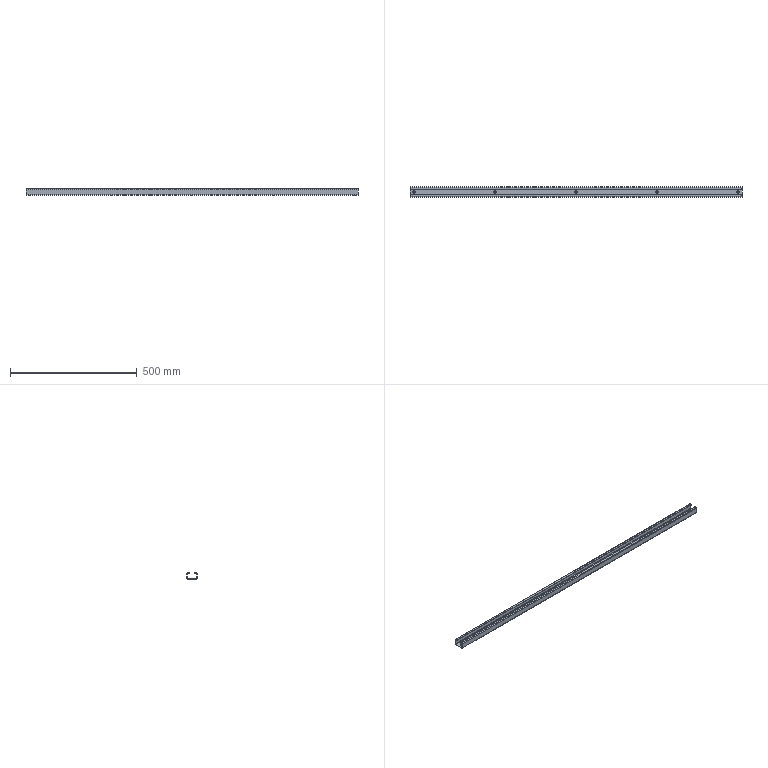Part | NX | features solid 2 | 1 solid | 36 faces | box 1310 x 39.5 x 25.5 mm | volume 197290 mm3 | plane 14 | cylinder 12 | cone 10 | commonest cylinder face diameters 3 x4 6 x4 10 x4
STEP:
#1=CARTESIAN_POINT('',(-273.5,-1500.5,1297.5));
#2=VERTEX_POINT('',#1);
#3=CARTESIAN_POINT('',(-268.5,-1505.5,1297.5));
#4=VERTEX_POINT('',#3);
#5=CARTESIAN_POINT('',(-268.5,-1500.5,1297.5));
#6=DIRECTION('',(0.,0.,1.));
#7=DIRECTION('',(0.,1.,0.));
#8=AXIS2_PLACEMENT_3D('',#5,#6,#7);
#9=CIRCLE('',#8,5.);
#10=EDGE_CURVE('',#2,#4,#9,.T.);
#11=ORIENTED_EDGE('',*,*,#10,.F.);
#12=CARTESIAN_POINT('',(-273.5,-1500.5,1296.));
#13=VERTEX_POINT('',#12);
#14=CARTESIAN_POINT('',(-273.5,-1500.5,1297.5));
#15=DIRECTION('',(0.,0.,1.));
#16=VECTOR('',#15,1000.);
#17=LINE('',#14,#16);
#18=EDGE_CURVE('',#13,#2,#17,.T.);
#19=ORIENTED_EDGE('',*,*,#18,.F.);
#20=CARTESIAN_POINT('',(-268.5,-1505.5,1296.));
#21=VERTEX_POINT('',#20);
#22=CARTESIAN_POINT('',(-268.5,-1500.5,1296.));
#23=DIRECTION('',(0.,0.,-1.));
#24=DIRECTION('',(0.,1.,0.));
#25=AXIS2_PLACEMENT_3D('',#22,#23,#24);
#26=CIRCLE('',#25,5.);
#27=EDGE_CURVE('',#21,#13,#26,.T.);
#28=ORIENTED_EDGE('',*,*,#27,.F.);
#29=CARTESIAN_POINT('',(-268.5,-1505.5,1297.5));
#30=DIRECTION('',(0.,0.,-1.));
#31=VECTOR('',#30,1000.);
#32=LINE('',#29,#31);
#33=EDGE_CURVE('',#4,#21,#32,.T.);
#34=ORIENTED_EDGE('',*,*,#33,.F.);
#35=EDGE_LOOP('',(#11,#19,#28,#34));
#36=FACE_BOUND('',#35,.T.);
#37=CARTESIAN_POINT('',(-268.5,-1500.5,1297.5));
#38=DIRECTION('',(0.,0.,1.));
#39=DIRECTION('',(0.,-1.,0.));
#40=AXIS2_PLACEMENT_3D('',#37,#38,#39);
#41=CYLINDRICAL_SURFACE('',#40,5.);
#42=ADVANCED_FACE('',(#36),#41,.T.);
#43=CARTESIAN_POINT('',(-268.5,-1525.,1297.5));
#44=VERTEX_POINT('',#43);
#45=CARTESIAN_POINT('',(-273.5,-1530.,1297.5));
#46=VERTEX_POINT('',#45);
#47=CARTESIAN_POINT('',(-268.5,-1530.,1297.5));
#48=DIRECTION('',(0.,0.,1.));
#49=DIRECTION('',(0.,1.,0.));
#50=AXIS2_PLACEMENT_3D('',#47,#48,#49);
#51=CIRCLE('',#50,5.);
#52=EDGE_CURVE('',#44,#46,#51,.T.);
#53=ORIENTED_EDGE('',*,*,#52,.F.);
#54=CARTESIAN_POINT('',(-268.5,-1525.,1296.));
#55=VERTEX_POINT('',#54);
#56=CARTESIAN_POINT('',(-268.5,-1525.,1297.5));
#57=DIRECTION('',(0.,0.,1.));
#58=VECTOR('',#57,1000.);
#59=LINE('',#56,#58);
#60=EDGE_CURVE('',#55,#44,#59,.T.);
#61=ORIENTED_EDGE('',*,*,#60,.F.);
#62=CARTESIAN_POINT('',(-273.5,-1530.,1296.));
#63=VERTEX_POINT('',#62);
#64=CARTESIAN_POINT('',(-268.5,-1530.,1296.));
#65=DIRECTION('',(0.,0.,-1.));
#66=DIRECTION('',(0.,1.,0.));
#67=AXIS2_PLACEMENT_3D('',#64,#65,#66);
#68=CIRCLE('',#67,5.);
#69=EDGE_CURVE('',#63,#55,#68,.T.);
#70=ORIENTED_EDGE('',*,*,#69,.F.);
#71=CARTESIAN_POINT('',(-273.5,-1530.,1297.5));
#72=DIRECTION('',(0.,0.,-1.));
#73=VECTOR('',#72,1000.);
#74=LINE('',#71,#73);
#75=EDGE_CURVE('',#46,#63,#74,.T.);
#76=ORIENTED_EDGE('',*,*,#75,.F.);
#77=EDGE_LOOP('',(#53,#61,#70,#76));
#78=FACE_BOUND('',#77,.T.);
#79=CARTESIAN_POINT('',(-268.5,-1530.,1297.5));
#80=DIRECTION('',(0.,0.,-1.));
#81=DIRECTION('',(0.,1.,0.));
#82=AXIS2_PLACEMENT_3D('',#79,#80,#81);
#83=CYLINDRICAL_SURFACE('',#82,5.);
#84=ADVANCED_FACE('',(#78),#83,.T.);
#85=CARTESIAN_POINT('',(1036.5,-1530.,1297.5));
#86=VERTEX_POINT('',#85);
#87=CARTESIAN_POINT('',(1031.5,-1525.,1297.5));
#88=VERTEX_POINT('',#87);
#89=CARTESIAN_POINT('',(1031.5,-1530.,1297.5));
#90=DIRECTION('',(0.,0.,1.));
#91=DIRECTION('',(0.,1.,0.));
#92=AXIS2_PLACEMENT_3D('',#89,#90,#91);
#93=CIRCLE('',#92,5.);
#94=EDGE_CURVE('',#86,#88,#93,.T.);
#95=ORIENTED_EDGE('',*,*,#94,.F.);
#96=CARTESIAN_POINT('',(1036.5,-1530.,1296.));
#97=VERTEX_POINT('',#96);
#98=CARTESIAN_POINT('',(1036.5,-1530.,1297.5));
#99=DIRECTION('',(0.,0.,1.));
#100=VECTOR('',#99,1000.);
#101=LINE('',#98,#100);
#102=EDGE_CURVE('',#97,#86,#101,.T.);
#103=ORIENTED_EDGE('',*,*,#102,.F.);
#104=CARTESIAN_POINT('',(1031.5,-1525.,1296.));
#105=VERTEX_POINT('',#104);
#106=CARTESIAN_POINT('',(1031.5,-1530.,1296.));
#107=DIRECTION('',(0.,0.,-1.));
#108=DIRECTION('',(0.,1.,0.));
#109=AXIS2_PLACEMENT_3D('',#106,#107,#108);
#110=CIRCLE('',#109,5.);
#111=EDGE_CURVE('',#105,#97,#110,.T.);
#112=ORIENTED_EDGE('',*,*,#111,.F.);
#113=CARTESIAN_POINT('',(1031.5,-1525.,1297.5));
#114=DIRECTION('',(0.,0.,-1.));
#115=VECTOR('',#114,1000.);
#116=LINE('',#113,#115);
#117=EDGE_CURVE('',#88,#105,#116,.T.);
#118=ORIENTED_EDGE('',*,*,#117,.F.);
#119=EDGE_LOOP('',(#95,#103,#112,#118));
#120=FACE_BOUND('',#119,.T.);
#121=CARTESIAN_POINT('',(1031.5,-1530.,1297.5));
#122=DIRECTION('',(0.,0.,1.));
#123=DIRECTION('',(0.,-1.,0.));
#124=AXIS2_PLACEMENT_3D('',#121,#122,#123);
#125=CYLINDRICAL_SURFACE('',#124,5.);
#126=ADVANCED_FACE('',(#120),#125,.T.);
#127=CARTESIAN_POINT('',(1031.5,-1505.5,1297.5));
#128=VERTEX_POINT('',#127);
#129=CARTESIAN_POINT('',(1036.5,-1500.5,1297.5));
#130=VERTEX_POINT('',#129);
#131=CARTESIAN_POINT('',(1031.5,-1500.5,1297.5));
#132=DIRECTION('',(0.,0.,1.));
#133=DIRECTION('',(0.,1.,0.));
#134=AXIS2_PLACEMENT_3D('',#131,#132,#133);
#135=CIRCLE('',#134,5.);
#136=EDGE_CURVE('',#128,#130,#135,.T.);
#137=ORIENTED_EDGE('',*,*,#136,.F.);
#138=CARTESIAN_POINT('',(1031.5,-1505.5,1296.));
#139=VERTEX_POINT('',#138);
#140=CARTESIAN_POINT('',(1031.5,-1505.5,1297.5));
#141=DIRECTION('',(0.,0.,1.));
#142=VECTOR('',#141,1000.);
#143=LINE('',#140,#142);
#144=EDGE_CURVE('',#139,#128,#143,.T.);
#145=ORIENTED_EDGE('',*,*,#144,.F.);
#146=CARTESIAN_POINT('',(1036.5,-1500.5,1296.));
#147=VERTEX_POINT('',#146);
#148=CARTESIAN_POINT('',(1031.5,-1500.5,1296.));
#149=DIRECTION('',(0.,0.,-1.));
#150=DIRECTION('',(0.,1.,0.));
#151=AXIS2_PLACEMENT_3D('',#148,#149,#150);
#152=CIRCLE('',#151,5.);
#153=EDGE_CURVE('',#147,#139,#152,.T.);
#154=ORIENTED_EDGE('',*,*,#153,.F.);
#155=CARTESIAN_POINT('',(1036.5,-1500.5,1297.5));
#156=DIRECTION('',(0.,0.,-1.));
#157=VECTOR('',#156,1000.);
#158=LINE('',#155,#157);
#159=EDGE_CURVE('',#130,#147,#158,.T.);
#160=ORIENTED_EDGE('',*,*,#159,.F.);
#161=EDGE_LOOP('',(#137,#145,#154,#160));
#162=FACE_BOUND('',#161,.T.);
#163=CARTESIAN_POINT('',(1031.5,-1500.5,1297.5));
#164=DIRECTION('',(0.,0.,-1.));
#165=DIRECTION('',(0.,1.,0.));
#166=AXIS2_PLACEMENT_3D('',#163,#164,#165);
#167=CYLINDRICAL_SURFACE('',#166,5.);
#168=ADVANCED_FACE('',(#162),#167,.T.);
#169=CARTESIAN_POINT('',(-258.5,-1510.25,1273.5));
#170=VERTEX_POINT('',#169);
#171=CARTESIAN_POINT('',(-258.5,-1511.75,1272.));
#172=VERTEX_POINT('',#171);
#173=CARTESIAN_POINT('',(-258.5,-1511.75,1272.));
#174=DIRECTION('',(0.,0.7071,0.7071));
#175=VECTOR('',#174,1000.);
#176=LINE('',#173,#175);
#177=EDGE_CURVE('',#170,#172,#176,.F.);
#178=ORIENTED_EDGE('',*,*,#177,.T.);
#179=CARTESIAN_POINT('',(-258.5,-1518.75,1272.));
#180=VERTEX_POINT('',#179);
#181=CARTESIAN_POINT('',(-258.5,-1515.25,1272.));
#182=DIRECTION('',(0.,0.,-1.));
#183=DIRECTION('',(1.,0.,0.));
#184=AXIS2_PLACEMENT_3D('',#181,#182,#183);
#185=CIRCLE('',#184,3.5);
#186=EDGE_CURVE('',#172,#180,#185,.T.);
#187=ORIENTED_EDGE('',*,*,#186,.T.);
#188=CARTESIAN_POINT('',(-258.5,-1520.25,1273.5));
#189=VERTEX_POINT('',#188);
#190=CARTESIAN_POINT('',(-258.5,-1518.75,1272.));
#191=DIRECTION('',(0.,-0.7071,0.7071));
#192=VECTOR('',#191,1000.);
#193=LINE('',#190,#192);
#194=EDGE_CURVE('',#180,#189,#193,.T.);
#195=ORIENTED_EDGE('',*,*,#194,.T.);
#196=CARTESIAN_POINT('',(-258.5,-1515.25,1273.5));
#197=DIRECTION('',(0.,0.,-1.));
#198=DIRECTION('',(0.,-1.,0.));
#199=AXIS2_PLACEMENT_3D('',#196,#197,#198);
#200=CIRCLE('',#199,5.);
#201=EDGE_CURVE('',#170,#189,#200,.T.);
#202=ORIENTED_EDGE('',*,*,#201,.F.);
#203=EDGE_LOOP('',(#178,#187,#195,#202));
#204=FACE_BOUND('',#203,.T.);
#205=CARTESIAN_POINT('',(-258.5,-1515.25,1272.));
#206=DIRECTION('',(0.,0.,1.));
#207=DIRECTION('',(0.,-1.,0.));
#208=AXIS2_PLACEMENT_3D('',#205,#206,#207);
#209=CONICAL_SURFACE('',#208,3.5,0.7854);
#210=ADVANCED_FACE('',(#204),#209,.F.);
#211=CARTESIAN_POINT('',(61.5,-1511.75,1272.));
#212=VERTEX_POINT('',#211);
#213=CARTESIAN_POINT('',(61.5,-1510.25,1273.5));
#214=VERTEX_POINT('',#213);
#215=CARTESIAN_POINT('',(61.5,-1511.75,1272.));
#216=DIRECTION('',(0.,0.7071,0.7071));
#217=VECTOR('',#216,1000.);
#218=LINE('',#215,#217);
#219=EDGE_CURVE('',#212,#214,#218,.T.);
#220=ORIENTED_EDGE('',*,*,#219,.F.);
#221=CARTESIAN_POINT('',(61.5,-1518.75,1272.));
#222=VERTEX_POINT('',#221);
#223=CARTESIAN_POINT('',(61.5,-1515.25,1272.));
#224=DIRECTION('',(0.,0.,-1.));
#225=DIRECTION('',(1.,0.,0.));
#226=AXIS2_PLACEMENT_3D('',#223,#224,#225);
#227=CIRCLE('',#226,3.5);
#228=EDGE_CURVE('',#212,#222,#227,.T.);
#229=ORIENTED_EDGE('',*,*,#228,.T.);
#230=CARTESIAN_POINT('',(61.5,-1520.25,1273.5));
#231=VERTEX_POINT('',#230);
#232=CARTESIAN_POINT('',(61.5,-1518.75,1272.));
#233=DIRECTION('',(0.,-0.7071,0.7071));
#234=VECTOR('',#233,1000.);
#235=LINE('',#232,#234);
#236=EDGE_CURVE('',#231,#222,#235,.F.);
#237=ORIENTED_EDGE('',*,*,#236,.F.);
#238=CARTESIAN_POINT('',(61.5,-1515.25,1273.5));
#239=DIRECTION('',(0.,0.,-1.));
#240=DIRECTION('',(0.,-1.,0.));
#241=AXIS2_PLACEMENT_3D('',#238,#239,#240);
#242=CIRCLE('',#241,5.);
#243=EDGE_CURVE('',#214,#231,#242,.T.);
#244=ORIENTED_EDGE('',*,*,#243,.F.);
#245=EDGE_LOOP('',(#220,#229,#237,#244));
#246=FACE_BOUND('',#245,.T.);
#247=CARTESIAN_POINT('',(61.5,-1515.25,1272.));
#248=DIRECTION('',(0.,0.,1.));
#249=DIRECTION('',(0.,-1.,0.));
#250=AXIS2_PLACEMENT_3D('',#247,#248,#249);
#251=CONICAL_SURFACE('',#250,3.5,0.7854);
#252=ADVANCED_FACE('',(#246),#251,.F.);
#253=CARTESIAN_POINT('',(381.5,-1511.75,1272.));
#254=VERTEX_POINT('',#253);
#255=CARTESIAN_POINT('',(381.5,-1510.25,1273.5));
#256=VERTEX_POINT('',#255);
#257=CARTESIAN_POINT('',(381.5,-1511.75,1272.));
#258=DIRECTION('',(0.,0.7071,0.7071));
#259=VECTOR('',#258,1000.);
#260=LINE('',#257,#259);
#261=EDGE_CURVE('',#254,#256,#260,.T.);
#262=ORIENTED_EDGE('',*,*,#261,.F.);
#263=CARTESIAN_POINT('',(381.5,-1518.75,1272.));
#264=VERTEX_POINT('',#263);
#265=CARTESIAN_POINT('',(381.5,-1515.25,1272.));
#266=DIRECTION('',(0.,0.,-1.));
#267=DIRECTION('',(1.,0.,0.));
#268=AXIS2_PLACEMENT_3D('',#265,#266,#267);
#269=CIRCLE('',#268,3.5);
#270=EDGE_CURVE('',#254,#264,#269,.T.);
#271=ORIENTED_EDGE('',*,*,#270,.T.);
#272=CARTESIAN_POINT('',(381.5,-1520.25,1273.5));
#273=VERTEX_POINT('',#272);
#274=CARTESIAN_POINT('',(381.5,-1518.75,1272.));
#275=DIRECTION('',(0.,-0.7071,0.7071));
#276=VECTOR('',#275,1000.);
#277=LINE('',#274,#276);
#278=EDGE_CURVE('',#273,#264,#277,.F.);
#279=ORIENTED_EDGE('',*,*,#278,.F.);
#280=CARTESIAN_POINT('',(381.5,-1515.25,1273.5));
#281=DIRECTION('',(0.,0.,-1.));
#282=DIRECTION('',(0.,-1.,0.));
#283=AXIS2_PLACEMENT_3D('',#280,#281,#282);
#284=CIRCLE('',#283,5.);
#285=EDGE_CURVE('',#256,#273,#284,.T.);
#286=ORIENTED_EDGE('',*,*,#285,.F.);
#287=EDGE_LOOP('',(#262,#271,#279,#286));
#288=FACE_BOUND('',#287,.T.);
#289=CARTESIAN_POINT('',(381.5,-1515.25,1272.));
#290=DIRECTION('',(0.,0.,1.));
#291=DIRECTION('',(0.,-1.,0.));
#292=AXIS2_PLACEMENT_3D('',#289,#290,#291);
#293=CONICAL_SURFACE('',#292,3.5,0.7854);
#294=ADVANCED_FACE('',(#288),#293,.F.);
#295=CARTESIAN_POINT('',(701.5,-1511.75,1272.));
#296=VERTEX_POINT('',#295);
#297=CARTESIAN_POINT('',(701.5,-1510.25,1273.5));
#298=VERTEX_POINT('',#297);
#299=CARTESIAN_POINT('',(701.5,-1511.75,1272.));
#300=DIRECTION('',(0.,0.7071,0.7071));
#301=VECTOR('',#300,1000.);
#302=LINE('',#299,#301);
#303=EDGE_CURVE('',#296,#298,#302,.T.);
#304=ORIENTED_EDGE('',*,*,#303,.F.);
#305=CARTESIAN_POINT('',(701.5,-1518.75,1272.));
#306=VERTEX_POINT('',#305);
#307=CARTESIAN_POINT('',(701.5,-1515.25,1272.));
#308=DIRECTION('',(0.,0.,-1.));
#309=DIRECTION('',(1.,0.,0.));
#310=AXIS2_PLACEMENT_3D('',#307,#308,#309);
#311=CIRCLE('',#310,3.5);
#312=EDGE_CURVE('',#296,#306,#311,.T.);
#313=ORIENTED_EDGE('',*,*,#312,.T.);
#314=CARTESIAN_POINT('',(701.5,-1520.25,1273.5));
#315=VERTEX_POINT('',#314);
#316=CARTESIAN_POINT('',(701.5,-1518.75,1272.));
#317=DIRECTION('',(0.,-0.7071,0.7071));
#318=VECTOR('',#317,1000.);
#319=LINE('',#316,#318);
#320=EDGE_CURVE('',#315,#306,#319,.F.);
#321=ORIENTED_EDGE('',*,*,#320,.F.);
#322=CARTESIAN_POINT('',(701.5,-1515.25,1273.5));
#323=DIRECTION('',(0.,0.,-1.));
#324=DIRECTION('',(0.,-1.,0.));
#325=AXIS2_PLACEMENT_3D('',#322,#323,#324);
#326=CIRCLE('',#325,5.);
#327=EDGE_CURVE('',#298,#315,#326,.T.);
#328=ORIENTED_EDGE('',*,*,#327,.F.);
#329=EDGE_LOOP('',(#304,#313,#321,#328));
#330=FACE_BOUND('',#329,.T.);
#331=CARTESIAN_POINT('',(701.5,-1515.25,1272.));
#332=DIRECTION('',(0.,0.,1.));
#333=DIRECTION('',(0.,-1.,0.));
#334=AXIS2_PLACEMENT_3D('',#331,#332,#333);
#335=CONICAL_SURFACE('',#334,3.5,0.7854);
#336=ADVANCED_FACE('',(#330),#335,.F.);
#337=CARTESIAN_POINT('',(1021.5,-1510.25,1273.5));
#338=VERTEX_POINT('',#337);
#339=CARTESIAN_POINT('',(1021.5,-1511.75,1272.));
#340=VERTEX_POINT('',#339);
#341=CARTESIAN_POINT('',(1021.5,-1511.75,1272.));
#342=DIRECTION('',(0.,0.7071,0.7071));
#343=VECTOR('',#342,1000.);
#344=LINE('',#341,#343);
#345=EDGE_CURVE('',#338,#340,#344,.F.);
#346=ORIENTED_EDGE('',*,*,#345,.T.);
#347=CARTESIAN_POINT('',(1021.5,-1518.75,1272.));
#348=VERTEX_POINT('',#347);
#349=CARTESIAN_POINT('',(1021.5,-1515.25,1272.));
#350=DIRECTION('',(0.,0.,-1.));
#351=DIRECTION('',(1.,0.,0.));
#352=AXIS2_PLACEMENT_3D('',#349,#350,#351);
#353=CIRCLE('',#352,3.5);
#354=EDGE_CURVE('',#340,#348,#353,.T.);
#355=ORIENTED_EDGE('',*,*,#354,.T.);
#356=CARTESIAN_POINT('',(1021.5,-1520.25,1273.5));
#357=VERTEX_POINT('',#356);
#358=CARTESIAN_POINT('',(1021.5,-1518.75,1272.));
#359=DIRECTION('',(0.,-0.7071,0.7071));
#360=VECTOR('',#359,1000.);
#361=LINE('',#358,#360);
#362=EDGE_CURVE('',#348,#357,#361,.T.);
#363=ORIENTED_EDGE('',*,*,#362,.T.);
#364=CARTESIAN_POINT('',(1021.5,-1515.25,1273.5));
#365=DIRECTION('',(0.,0.,-1.));
#366=DIRECTION('',(0.,-1.,0.));
#367=AXIS2_PLACEMENT_3D('',#364,#365,#366);
#368=CIRCLE('',#367,5.);
#369=EDGE_CURVE('',#338,#357,#368,.T.);
#370=ORIENTED_EDGE('',*,*,#369,.F.);
#371=EDGE_LOOP('',(#346,#355,#363,#370));
#372=FACE_BOUND('',#371,.T.);
#373=CARTESIAN_POINT('',(1021.5,-1515.25,1272.));
#374=DIRECTION('',(0.,0.,1.));
#375=DIRECTION('',(0.,-1.,0.));
#376=AXIS2_PLACEMENT_3D('',#373,#374,#375);
#377=CONICAL_SURFACE('',#376,3.5,0.7854);
#378=ADVANCED_FACE('',(#372),#377,.F.);
#379=CARTESIAN_POINT('',(1036.5,-1505.5,1297.5));
#380=DIRECTION('',(-1.,0.,0.));
#381=VECTOR('',#380,1000.);
#382=LINE('',#379,#381);
#383=EDGE_CURVE('',#128,#4,#382,.T.);
#384=ORIENTED_EDGE('',*,*,#383,.F.);
#385=ORIENTED_EDGE('',*,*,#136,.T.);
#386=CARTESIAN_POINT('',(1036.5,-1498.5,1297.5));
#387=VERTEX_POINT('',#386);
#388=CARTESIAN_POINT('',(1036.5,-1495.5,1297.5));
#389=DIRECTION('',(0.,-1.,0.));
#390=VECTOR('',#389,1000.);
#391=LINE('',#388,#390);
#392=EDGE_CURVE('',#387,#130,#391,.T.);
#393=ORIENTED_EDGE('',*,*,#392,.F.);
#394=CARTESIAN_POINT('',(-273.5,-1498.5,1297.5));
#395=VERTEX_POINT('',#394);
#396=CARTESIAN_POINT('',(1036.5,-1498.5,1297.5));
#397=DIRECTION('',(-1.,0.,0.));
#398=VECTOR('',#397,1000.);
#399=LINE('',#396,#398);
#400=EDGE_CURVE('',#387,#395,#399,.T.);
#401=ORIENTED_EDGE('',*,*,#400,.T.);
#402=CARTESIAN_POINT('',(-273.5,-1495.5,1297.5));
#403=DIRECTION('',(0.,-1.,0.));
#404=VECTOR('',#403,1000.);
#405=LINE('',#402,#404);
#406=EDGE_CURVE('',#395,#2,#405,.T.);
#407=ORIENTED_EDGE('',*,*,#406,.T.);
#408=ORIENTED_EDGE('',*,*,#10,.T.);
#409=EDGE_LOOP('',(#384,#385,#393,#401,#407,#408));
#410=FACE_BOUND('',#409,.T.);
#411=CARTESIAN_POINT('',(1036.5,-1495.5,1297.5));
#412=DIRECTION('',(0.,0.,-1.));
#413=DIRECTION('',(0.,-1.,0.));
#414=AXIS2_PLACEMENT_3D('',#411,#412,#413);
#415=PLANE('',#414);
#416=ADVANCED_FACE('',(#410),#415,.F.);
#417=CARTESIAN_POINT('',(-273.5,-1495.5,1294.5));
#418=VERTEX_POINT('',#417);
#419=CARTESIAN_POINT('',(-273.5,-1498.5,1294.5));
#420=DIRECTION('',(1.,0.,0.));
#421=DIRECTION('',(0.,0.,1.));
#422=AXIS2_PLACEMENT_3D('',#419,#420,#421);
#423=CIRCLE('',#422,3.);
#424=EDGE_CURVE('',#418,#395,#423,.T.);
#425=ORIENTED_EDGE('',*,*,#424,.T.);
#426=ORIENTED_EDGE('',*,*,#400,.F.);
#427=CARTESIAN_POINT('',(1036.5,-1495.5,1294.5));
#428=VERTEX_POINT('',#427);
#429=CARTESIAN_POINT('',(1036.5,-1498.5,1294.5));
#430=DIRECTION('',(1.,0.,0.));
#431=DIRECTION('',(0.,0.,1.));
#432=AXIS2_PLACEMENT_3D('',#429,#430,#431);
#433=CIRCLE('',#432,3.);
#434=EDGE_CURVE('',#428,#387,#433,.T.);
#435=ORIENTED_EDGE('',*,*,#434,.F.);
#436=CARTESIAN_POINT('',(1036.5,-1495.5,1294.5));
#437=DIRECTION('',(-1.,0.,0.));
#438=VECTOR('',#437,1000.);
#439=LINE('',#436,#438);
#440=EDGE_CURVE('',#428,#418,#439,.T.);
#441=ORIENTED_EDGE('',*,*,#440,.T.);
#442=EDGE_LOOP('',(#425,#426,#435,#441));
#443=FACE_BOUND('',#442,.T.);
#444=CARTESIAN_POINT('',(1036.5,-1498.5,1294.5));
#445=DIRECTION('',(-1.,0.,0.));
#446=DIRECTION('',(0.,0.,1.));
#447=AXIS2_PLACEMENT_3D('',#444,#445,#446);
#448=CYLINDRICAL_SURFACE('',#447,3.);
#449=ADVANCED_FACE('',(#443),#448,.T.);
#450=CARTESIAN_POINT('',(-273.5,-1495.5,1275.));
#451=VERTEX_POINT('',#450);
#452=CARTESIAN_POINT('',(-273.5,-1495.5,1272.));
#453=DIRECTION('',(0.,0.,1.));
#454=VECTOR('',#453,1000.);
#455=LINE('',#452,#454);
#456=EDGE_CURVE('',#451,#418,#455,.T.);
#457=ORIENTED_EDGE('',*,*,#456,.T.);
#458=ORIENTED_EDGE('',*,*,#440,.F.);
#459=CARTESIAN_POINT('',(1036.5,-1495.5,1275.));
#460=VERTEX_POINT('',#459);
#461=CARTESIAN_POINT('',(1036.5,-1495.5,1272.));
#462=DIRECTION('',(0.,0.,1.));
#463=VECTOR('',#462,1000.);
#464=LINE('',#461,#463);
#465=EDGE_CURVE('',#460,#428,#464,.T.);
#466=ORIENTED_EDGE('',*,*,#465,.F.);
#467=CARTESIAN_POINT('',(1036.5,-1495.5,1275.));
#468=DIRECTION('',(-1.,0.,0.));
#469=VECTOR('',#468,1000.);
#470=LINE('',#467,#469);
#471=EDGE_CURVE('',#460,#451,#470,.T.);
#472=ORIENTED_EDGE('',*,*,#471,.T.);
#473=EDGE_LOOP('',(#457,#458,#466,#472));
#474=FACE_BOUND('',#473,.T.);
#475=CARTESIAN_POINT('',(1036.5,-1495.5,1272.));
#476=DIRECTION('',(0.,-1.,0.));
#477=DIRECTION('',(-1.,0.,0.));
#478=AXIS2_PLACEMENT_3D('',#475,#476,#477);
#479=PLANE('',#478);
#480=ADVANCED_FACE('',(#474),#479,.F.);
#481=CARTESIAN_POINT('',(-273.5,-1498.5,1272.));
#482=VERTEX_POINT('',#481);
#483=CARTESIAN_POINT('',(-273.5,-1498.5,1275.));
#484=DIRECTION('',(1.,0.,0.));
#485=DIRECTION('',(0.,0.,1.));
#486=AXIS2_PLACEMENT_3D('',#483,#484,#485);
#487=CIRCLE('',#486,3.);
#488=EDGE_CURVE('',#482,#451,#487,.T.);
#489=ORIENTED_EDGE('',*,*,#488,.T.);
#490=ORIENTED_EDGE('',*,*,#471,.F.);
#491=CARTESIAN_POINT('',(1036.5,-1498.5,1272.));
#492=VERTEX_POINT('',#491);
#493=CARTESIAN_POINT('',(1036.5,-1498.5,1275.));
#494=DIRECTION('',(1.,0.,0.));
#495=DIRECTION('',(0.,0.,1.));
#496=AXIS2_PLACEMENT_3D('',#493,#494,#495);
#497=CIRCLE('',#496,3.);
#498=EDGE_CURVE('',#492,#460,#497,.T.);
#499=ORIENTED_EDGE('',*,*,#498,.F.);
#500=CARTESIAN_POINT('',(1036.5,-1498.5,1272.));
#501=DIRECTION('',(-1.,0.,0.));
#502=VECTOR('',#501,1000.);
#503=LINE('',#500,#502);
#504=EDGE_CURVE('',#492,#482,#503,.T.);
#505=ORIENTED_EDGE('',*,*,#504,.T.);
#506=EDGE_LOOP('',(#489,#490,#499,#505));
#507=FACE_BOUND('',#506,.T.);
#508=CARTESIAN_POINT('',(1036.5,-1498.5,1275.));
#509=DIRECTION('',(-1.,0.,0.));
#510=DIRECTION('',(0.,0.,1.));
#511=AXIS2_PLACEMENT_3D('',#508,#509,#510);
#512=CYLINDRICAL_SURFACE('',#511,3.);
#513=ADVANCED_FACE('',(#507),#512,.T.);
#514=CARTESIAN_POINT('',(61.5,-1515.25,1272.));
#515=DIRECTION('',(0.,0.,-1.));
#516=DIRECTION('',(1.,0.,0.));
#517=AXIS2_PLACEMENT_3D('',#514,#515,#516);
#518=CIRCLE('',#517,3.5);
#519=EDGE_CURVE('',#222,#212,#518,.T.);
#520=ORIENTED_EDGE('',*,*,#519,.F.);
#521=ORIENTED_EDGE('',*,*,#228,.F.);
#522=EDGE_LOOP('',(#520,#521));
#523=FACE_BOUND('',#522,.T.);
#524=CARTESIAN_POINT('',(381.5,-1515.25,1272.));
#525=DIRECTION('',(0.,0.,-1.));
#526=DIRECTION('',(1.,0.,0.));
#527=AXIS2_PLACEMENT_3D('',#524,#525,#526);
#528=CIRCLE('',#527,3.5);
#529=EDGE_CURVE('',#264,#254,#528,.T.);
#530=ORIENTED_EDGE('',*,*,#529,.F.);
#531=ORIENTED_EDGE('',*,*,#270,.F.);
#532=EDGE_LOOP('',(#530,#531));
#533=FACE_BOUND('',#532,.T.);
#534=CARTESIAN_POINT('',(701.5,-1515.25,1272.));
#535=DIRECTION('',(0.,0.,-1.));
#536=DIRECTION('',(1.,0.,0.));
#537=AXIS2_PLACEMENT_3D('',#534,#535,#536);
#538=CIRCLE('',#537,3.5);
#539=EDGE_CURVE('',#306,#296,#538,.T.);
#540=ORIENTED_EDGE('',*,*,#539,.F.);
#541=ORIENTED_EDGE('',*,*,#312,.F.);
#542=EDGE_LOOP('',(#540,#541));
#543=FACE_BOUND('',#542,.T.);
#544=CARTESIAN_POINT('',(1021.5,-1515.25,1272.));
#545=DIRECTION('',(0.,0.,-1.));
#546=DIRECTION('',(1.,0.,0.));
#547=AXIS2_PLACEMENT_3D('',#544,#545,#546);
#548=CIRCLE('',#547,3.5);
#549=EDGE_CURVE('',#348,#340,#548,.T.);
#550=ORIENTED_EDGE('',*,*,#549,.F.);
#551=ORIENTED_EDGE('',*,*,#354,.F.);
#552=EDGE_LOOP('',(#550,#551));
#553=FACE_BOUND('',#552,.T.);
#554=CARTESIAN_POINT('',(-258.5,-1515.25,1272.));
#555=DIRECTION('',(0.,0.,-1.));
#556=DIRECTION('',(1.,0.,0.));
#557=AXIS2_PLACEMENT_3D('',#554,#555,#556);
#558=CIRCLE('',#557,3.5);
#559=EDGE_CURVE('',#180,#172,#558,.T.);
#560=ORIENTED_EDGE('',*,*,#559,.F.);
#561=ORIENTED_EDGE('',*,*,#186,.F.);
#562=EDGE_LOOP('',(#560,#561));
#563=FACE_BOUND('',#562,.T.);
#564=CARTESIAN_POINT('',(-273.5,-1532.,1272.));
#565=VERTEX_POINT('',#564);
#566=CARTESIAN_POINT('',(-273.5,-1535.,1272.));
#567=DIRECTION('',(0.,1.,0.));
#568=VECTOR('',#567,1000.);
#569=LINE('',#566,#568);
#570=EDGE_CURVE('',#565,#482,#569,.T.);
#571=ORIENTED_EDGE('',*,*,#570,.T.);
#572=ORIENTED_EDGE('',*,*,#504,.F.);
#573=CARTESIAN_POINT('',(1036.5,-1532.,1272.));
#574=VERTEX_POINT('',#573);
#575=CARTESIAN_POINT('',(1036.5,-1535.,1272.));
#576=DIRECTION('',(0.,1.,0.));
#577=VECTOR('',#576,1000.);
#578=LINE('',#575,#577);
#579=EDGE_CURVE('',#574,#492,#578,.T.);
#580=ORIENTED_EDGE('',*,*,#579,.F.);
#581=CARTESIAN_POINT('',(1036.5,-1532.,1272.));
#582=DIRECTION('',(-1.,0.,0.));
#583=VECTOR('',#582,1000.);
#584=LINE('',#581,#583);
#585=EDGE_CURVE('',#574,#565,#584,.T.);
#586=ORIENTED_EDGE('',*,*,#585,.T.);
#587=EDGE_LOOP('',(#571,#572,#580,#586));
#588=FACE_BOUND('',#587,.T.);
#589=CARTESIAN_POINT('',(1036.5,-1535.,1272.));
#590=DIRECTION('',(0.,0.,1.));
#591=DIRECTION('',(1.,0.,0.));
#592=AXIS2_PLACEMENT_3D('',#589,#590,#591);
#593=PLANE('',#592);
#594=ADVANCED_FACE('',(#523,#533,#543,#553,#563,#588),#593,.F.);
#595=CARTESIAN_POINT('',(-273.5,-1535.,1275.));
#596=VERTEX_POINT('',#595);
#597=CARTESIAN_POINT('',(-273.5,-1532.,1275.));
#598=DIRECTION('',(1.,0.,0.));
#599=DIRECTION('',(0.,0.,1.));
#600=AXIS2_PLACEMENT_3D('',#597,#598,#599);
#601=CIRCLE('',#600,3.);
#602=EDGE_CURVE('',#596,#565,#601,.T.);
#603=ORIENTED_EDGE('',*,*,#602,.T.);
#604=ORIENTED_EDGE('',*,*,#585,.F.);
#605=CARTESIAN_POINT('',(1036.5,-1535.,1275.));
#606=VERTEX_POINT('',#605);
#607=CARTESIAN_POINT('',(1036.5,-1532.,1275.));
#608=DIRECTION('',(1.,0.,0.));
#609=DIRECTION('',(0.,0.,1.));
#610=AXIS2_PLACEMENT_3D('',#607,#608,#609);
#611=CIRCLE('',#610,3.);
#612=EDGE_CURVE('',#606,#574,#611,.T.);
#613=ORIENTED_EDGE('',*,*,#612,.F.);
#614=CARTESIAN_POINT('',(1036.5,-1535.,1275.));
#615=DIRECTION('',(-1.,0.,0.));
#616=VECTOR('',#615,1000.);
#617=LINE('',#614,#616);
#618=EDGE_CURVE('',#606,#596,#617,.T.);
#619=ORIENTED_EDGE('',*,*,#618,.T.);
#620=EDGE_LOOP('',(#603,#604,#613,#619));
#621=FACE_BOUND('',#620,.T.);
#622=CARTESIAN_POINT('',(1036.5,-1532.,1275.));
#623=DIRECTION('',(-1.,0.,0.));
#624=DIRECTION('',(0.,0.,1.));
#625=AXIS2_PLACEMENT_3D('',#622,#623,#624);
#626=CYLINDRICAL_SURFACE('',#625,3.);
#627=ADVANCED_FACE('',(#621),#626,.T.);
#628=CARTESIAN_POINT('',(-273.5,-1535.,1294.5));
#629=VERTEX_POINT('',#628);
#630=CARTESIAN_POINT('',(-273.5,-1535.,1297.5));
#631=DIRECTION('',(0.,0.,-1.));
#632=VECTOR('',#631,1000.);
#633=LINE('',#630,#632);
#634=EDGE_CURVE('',#629,#596,#633,.T.);
#635=ORIENTED_EDGE('',*,*,#634,.T.);
#636=ORIENTED_EDGE('',*,*,#618,.F.);
#637=CARTESIAN_POINT('',(1036.5,-1535.,1294.5));
#638=VERTEX_POINT('',#637);
#639=CARTESIAN_POINT('',(1036.5,-1535.,1297.5));
#640=DIRECTION('',(0.,0.,-1.));
#641=VECTOR('',#640,1000.);
#642=LINE('',#639,#641);
#643=EDGE_CURVE('',#638,#606,#642,.T.);
#644=ORIENTED_EDGE('',*,*,#643,.F.);
#645=CARTESIAN_POINT('',(1036.5,-1535.,1294.5));
#646=DIRECTION('',(-1.,0.,0.));
#647=VECTOR('',#646,1000.);
#648=LINE('',#645,#647);
#649=EDGE_CURVE('',#638,#629,#648,.T.);
#650=ORIENTED_EDGE('',*,*,#649,.T.);
#651=EDGE_LOOP('',(#635,#636,#644,#650));
#652=FACE_BOUND('',#651,.T.);
#653=CARTESIAN_POINT('',(1036.5,-1535.,1297.5));
#654=DIRECTION('',(0.,1.,0.));
#655=DIRECTION('',(0.,0.,-1.));
#656=AXIS2_PLACEMENT_3D('',#653,#654,#655);
#657=PLANE('',#656);
#658=ADVANCED_FACE('',(#652),#657,.F.);
#659=CARTESIAN_POINT('',(-273.5,-1532.,1297.5));
#660=VERTEX_POINT('',#659);
#661=CARTESIAN_POINT('',(-273.5,-1532.,1294.5));
#662=DIRECTION('',(1.,0.,0.));
#663=DIRECTION('',(0.,0.,1.));
#664=AXIS2_PLACEMENT_3D('',#661,#662,#663);
#665=CIRCLE('',#664,3.);
#666=EDGE_CURVE('',#660,#629,#665,.T.);
#667=ORIENTED_EDGE('',*,*,#666,.T.);
#668=ORIENTED_EDGE('',*,*,#649,.F.);
#669=CARTESIAN_POINT('',(1036.5,-1532.,1297.5));
#670=VERTEX_POINT('',#669);
#671=CARTESIAN_POINT('',(1036.5,-1532.,1294.5));
#672=DIRECTION('',(1.,0.,0.));
#673=DIRECTION('',(0.,0.,1.));
#674=AXIS2_PLACEMENT_3D('',#671,#672,#673);
#675=CIRCLE('',#674,3.);
#676=EDGE_CURVE('',#670,#638,#675,.T.);
#677=ORIENTED_EDGE('',*,*,#676,.F.);
#678=CARTESIAN_POINT('',(1036.5,-1532.,1297.5));
#679=DIRECTION('',(-1.,0.,0.));
#680=VECTOR('',#679,1000.);
#681=LINE('',#678,#680);
#682=EDGE_CURVE('',#670,#660,#681,.T.);
#683=ORIENTED_EDGE('',*,*,#682,.T.);
#684=EDGE_LOOP('',(#667,#668,#677,#683));
#685=FACE_BOUND('',#684,.T.);
#686=CARTESIAN_POINT('',(1036.5,-1532.,1294.5));
#687=DIRECTION('',(-1.,0.,0.));
#688=DIRECTION('',(0.,0.,1.));
#689=AXIS2_PLACEMENT_3D('',#686,#687,#688);
#690=CYLINDRICAL_SURFACE('',#689,3.);
#691=ADVANCED_FACE('',(#685),#690,.T.);
#692=CARTESIAN_POINT('',(1036.5,-1525.,1297.5));
#693=DIRECTION('',(0.,-1.,0.));
#694=VECTOR('',#693,1000.);
#695=LINE('',#692,#694);
#696=EDGE_CURVE('',#86,#670,#695,.T.);
#697=ORIENTED_EDGE('',*,*,#696,.F.);
#698=ORIENTED_EDGE('',*,*,#94,.T.);
#699=CARTESIAN_POINT('',(1036.5,-1525.,1297.5));
#700=DIRECTION('',(-1.,0.,0.));
#701=VECTOR('',#700,1000.);
#702=LINE('',#699,#701);
#703=EDGE_CURVE('',#88,#44,#702,.T.);
#704=ORIENTED_EDGE('',*,*,#703,.T.);
#705=ORIENTED_EDGE('',*,*,#52,.T.);
#706=CARTESIAN_POINT('',(-273.5,-1525.,1297.5));
#707=DIRECTION('',(0.,-1.,0.));
#708=VECTOR('',#707,1000.);
#709=LINE('',#706,#708);
#710=EDGE_CURVE('',#46,#660,#709,.T.);
#711=ORIENTED_EDGE('',*,*,#710,.T.);
#712=ORIENTED_EDGE('',*,*,#682,.F.);
#713=EDGE_LOOP('',(#697,#698,#704,#705,#711,#712));
#714=FACE_BOUND('',#713,.T.);
#715=CARTESIAN_POINT('',(1036.5,-1525.,1297.5));
#716=DIRECTION('',(0.,0.,-1.));
#717=DIRECTION('',(0.,-1.,0.));
#718=AXIS2_PLACEMENT_3D('',#715,#716,#717);
#719=PLANE('',#718);
#720=ADVANCED_FACE('',(#714),#719,.F.);
#721=CARTESIAN_POINT('',(1036.5,-1498.5,1296.));
#722=VERTEX_POINT('',#721);
#723=CARTESIAN_POINT('',(1036.5,-1495.5,1296.));
#724=DIRECTION('',(0.,-1.,0.));
#725=VECTOR('',#724,1000.);
#726=LINE('',#723,#725);
#727=EDGE_CURVE('',#722,#147,#726,.T.);
#728=ORIENTED_EDGE('',*,*,#727,.T.);
#729=ORIENTED_EDGE('',*,*,#153,.T.);
#730=CARTESIAN_POINT('',(1036.5,-1505.5,1296.));
#731=DIRECTION('',(-1.,0.,0.));
#732=VECTOR('',#731,1000.);
#733=LINE('',#730,#732);
#734=EDGE_CURVE('',#139,#21,#733,.T.);
#735=ORIENTED_EDGE('',*,*,#734,.T.);
#736=ORIENTED_EDGE('',*,*,#27,.T.);
#737=CARTESIAN_POINT('',(-273.5,-1498.5,1296.));
#738=VERTEX_POINT('',#737);
#739=CARTESIAN_POINT('',(-273.5,-1495.5,1296.));
#740=DIRECTION('',(0.,-1.,0.));
#741=VECTOR('',#740,1000.);
#742=LINE('',#739,#741);
#743=EDGE_CURVE('',#738,#13,#742,.T.);
#744=ORIENTED_EDGE('',*,*,#743,.F.);
#745=CARTESIAN_POINT('',(1036.5,-1498.5,1296.));
#746=DIRECTION('',(-1.,0.,0.));
#747=VECTOR('',#746,1000.);
#748=LINE('',#745,#747);
#749=EDGE_CURVE('',#722,#738,#748,.T.);
#750=ORIENTED_EDGE('',*,*,#749,.F.);
#751=EDGE_LOOP('',(#728,#729,#735,#736,#744,#750));
#752=FACE_BOUND('',#751,.T.);
#753=CARTESIAN_POINT('',(1036.5,-1495.5,1296.));
#754=DIRECTION('',(0.,0.,-1.));
#755=DIRECTION('',(0.,-1.,0.));
#756=AXIS2_PLACEMENT_3D('',#753,#754,#755);
#757=PLANE('',#756);
#758=ADVANCED_FACE('',(#752),#757,.T.);
#759=CARTESIAN_POINT('',(-273.5,-1497.,1294.5));
#760=VERTEX_POINT('',#759);
#761=CARTESIAN_POINT('',(-273.5,-1498.5,1294.5));
#762=DIRECTION('',(1.,0.,0.));
#763=DIRECTION('',(0.,0.,1.));
#764=AXIS2_PLACEMENT_3D('',#761,#762,#763);
#765=CIRCLE('',#764,1.5);
#766=EDGE_CURVE('',#760,#738,#765,.T.);
#767=ORIENTED_EDGE('',*,*,#766,.F.);
#768=CARTESIAN_POINT('',(1036.5,-1497.,1294.5));
#769=VERTEX_POINT('',#768);
#770=CARTESIAN_POINT('',(1036.5,-1497.,1294.5));
#771=DIRECTION('',(-1.,0.,0.));
#772=VECTOR('',#771,1000.);
#773=LINE('',#770,#772);
#774=EDGE_CURVE('',#769,#760,#773,.T.);
#775=ORIENTED_EDGE('',*,*,#774,.F.);
#776=CARTESIAN_POINT('',(1036.5,-1498.5,1294.5));
#777=DIRECTION('',(1.,0.,0.));
#778=DIRECTION('',(0.,0.,1.));
#779=AXIS2_PLACEMENT_3D('',#776,#777,#778);
#780=CIRCLE('',#779,1.5);
#781=EDGE_CURVE('',#769,#722,#780,.T.);
#782=ORIENTED_EDGE('',*,*,#781,.T.);
#783=ORIENTED_EDGE('',*,*,#749,.T.);
#784=EDGE_LOOP('',(#767,#775,#782,#783));
#785=FACE_BOUND('',#784,.T.);
#786=CARTESIAN_POINT('',(1036.5,-1498.5,1294.5));
#787=DIRECTION('',(-1.,0.,0.));
#788=DIRECTION('',(0.,0.,1.));
#789=AXIS2_PLACEMENT_3D('',#786,#787,#788);
#790=CYLINDRICAL_SURFACE('',#789,1.5);
#791=ADVANCED_FACE('',(#785),#790,.F.);
#792=CARTESIAN_POINT('',(-273.5,-1497.,1275.));
#793=VERTEX_POINT('',#792);
#794=CARTESIAN_POINT('',(-273.5,-1497.,1272.));
#795=DIRECTION('',(0.,0.,1.));
#796=VECTOR('',#795,1000.);
#797=LINE('',#794,#796);
#798=EDGE_CURVE('',#793,#760,#797,.T.);
#799=ORIENTED_EDGE('',*,*,#798,.F.);
#800=CARTESIAN_POINT('',(1036.5,-1497.,1275.));
#801=VERTEX_POINT('',#800);
#802=CARTESIAN_POINT('',(1036.5,-1497.,1275.));
#803=DIRECTION('',(-1.,0.,0.));
#804=VECTOR('',#803,1000.);
#805=LINE('',#802,#804);
#806=EDGE_CURVE('',#801,#793,#805,.T.);
#807=ORIENTED_EDGE('',*,*,#806,.F.);
#808=CARTESIAN_POINT('',(1036.5,-1497.,1272.));
#809=DIRECTION('',(0.,0.,1.));
#810=VECTOR('',#809,1000.);
#811=LINE('',#808,#810);
#812=EDGE_CURVE('',#801,#769,#811,.T.);
#813=ORIENTED_EDGE('',*,*,#812,.T.);
#814=ORIENTED_EDGE('',*,*,#774,.T.);
#815=EDGE_LOOP('',(#799,#807,#813,#814));
#816=FACE_BOUND('',#815,.T.);
#817=CARTESIAN_POINT('',(1036.5,-1497.,1272.));
#818=DIRECTION('',(0.,-1.,0.));
#819=DIRECTION('',(-1.,0.,0.));
#820=AXIS2_PLACEMENT_3D('',#817,#818,#819);
#821=PLANE('',#820);
#822=ADVANCED_FACE('',(#816),#821,.T.);
#823=CARTESIAN_POINT('',(-273.5,-1498.5,1273.5));
#824=VERTEX_POINT('',#823);
#825=CARTESIAN_POINT('',(-273.5,-1498.5,1275.));
#826=DIRECTION('',(1.,0.,0.));
#827=DIRECTION('',(0.,0.,1.));
#828=AXIS2_PLACEMENT_3D('',#825,#826,#827);
#829=CIRCLE('',#828,1.5);
#830=EDGE_CURVE('',#824,#793,#829,.T.);
#831=ORIENTED_EDGE('',*,*,#830,.F.);
#832=CARTESIAN_POINT('',(1036.5,-1498.5,1273.5));
#833=VERTEX_POINT('',#832);
#834=CARTESIAN_POINT('',(1036.5,-1498.5,1273.5));
#835=DIRECTION('',(-1.,0.,0.));
#836=VECTOR('',#835,1000.);
#837=LINE('',#834,#836);
#838=EDGE_CURVE('',#833,#824,#837,.T.);
#839=ORIENTED_EDGE('',*,*,#838,.F.);
#840=CARTESIAN_POINT('',(1036.5,-1498.5,1275.));
#841=DIRECTION('',(1.,0.,0.));
#842=DIRECTION('',(0.,0.,1.));
#843=AXIS2_PLACEMENT_3D('',#840,#841,#842);
#844=CIRCLE('',#843,1.5);
#845=EDGE_CURVE('',#833,#801,#844,.T.);
#846=ORIENTED_EDGE('',*,*,#845,.T.);
#847=ORIENTED_EDGE('',*,*,#806,.T.);
#848=EDGE_LOOP('',(#831,#839,#846,#847));
#849=FACE_BOUND('',#848,.T.);
#850=CARTESIAN_POINT('',(1036.5,-1498.5,1275.));
#851=DIRECTION('',(-1.,0.,0.));
#852=DIRECTION('',(0.,0.,1.));
#853=AXIS2_PLACEMENT_3D('',#850,#851,#852);
#854=CYLINDRICAL_SURFACE('',#853,1.5);
#855=ADVANCED_FACE('',(#849),#854,.F.);
#856=CARTESIAN_POINT('',(-258.5,-1515.25,1273.5));
#857=DIRECTION('',(0.,0.,-1.));
#858=DIRECTION('',(0.,-1.,0.));
#859=AXIS2_PLACEMENT_3D('',#856,#857,#858);
#860=CIRCLE('',#859,5.);
#861=EDGE_CURVE('',#189,#170,#860,.T.);
#862=ORIENTED_EDGE('',*,*,#861,.T.);
#863=ORIENTED_EDGE('',*,*,#201,.T.);
#864=EDGE_LOOP('',(#862,#863));
#865=FACE_BOUND('',#864,.T.);
#866=CARTESIAN_POINT('',(61.5,-1515.25,1273.5));
#867=DIRECTION('',(0.,0.,-1.));
#868=DIRECTION('',(0.,-1.,0.));
#869=AXIS2_PLACEMENT_3D('',#866,#867,#868);
#870=CIRCLE('',#869,5.);
#871=EDGE_CURVE('',#231,#214,#870,.T.);
#872=ORIENTED_EDGE('',*,*,#871,.T.);
#873=ORIENTED_EDGE('',*,*,#243,.T.);
#874=EDGE_LOOP('',(#872,#873));
#875=FACE_BOUND('',#874,.T.);
#876=CARTESIAN_POINT('',(381.5,-1515.25,1273.5));
#877=DIRECTION('',(0.,0.,-1.));
#878=DIRECTION('',(0.,-1.,0.));
#879=AXIS2_PLACEMENT_3D('',#876,#877,#878);
#880=CIRCLE('',#879,5.);
#881=EDGE_CURVE('',#273,#256,#880,.T.);
#882=ORIENTED_EDGE('',*,*,#881,.T.);
#883=ORIENTED_EDGE('',*,*,#285,.T.);
#884=EDGE_LOOP('',(#882,#883));
#885=FACE_BOUND('',#884,.T.);
#886=CARTESIAN_POINT('',(701.5,-1515.25,1273.5));
#887=DIRECTION('',(0.,0.,-1.));
#888=DIRECTION('',(0.,-1.,0.));
#889=AXIS2_PLACEMENT_3D('',#886,#887,#888);
#890=CIRCLE('',#889,5.);
#891=EDGE_CURVE('',#315,#298,#890,.T.);
#892=ORIENTED_EDGE('',*,*,#891,.T.);
#893=ORIENTED_EDGE('',*,*,#327,.T.);
#894=EDGE_LOOP('',(#892,#893));
#895=FACE_BOUND('',#894,.T.);
#896=CARTESIAN_POINT('',(1021.5,-1515.25,1273.5));
#897=DIRECTION('',(0.,0.,-1.));
#898=DIRECTION('',(0.,-1.,0.));
#899=AXIS2_PLACEMENT_3D('',#896,#897,#898);
#900=CIRCLE('',#899,5.);
#901=EDGE_CURVE('',#357,#338,#900,.T.);
#902=ORIENTED_EDGE('',*,*,#901,.T.);
#903=ORIENTED_EDGE('',*,*,#369,.T.);
#904=EDGE_LOOP('',(#902,#903));
#905=FACE_BOUND('',#904,.T.);
#906=CARTESIAN_POINT('',(-273.5,-1532.,1273.5));
#907=VERTEX_POINT('',#906);
#908=CARTESIAN_POINT('',(-273.5,-1535.,1273.5));
#909=DIRECTION('',(0.,1.,0.));
#910=VECTOR('',#909,1000.);
#911=LINE('',#908,#910);
#912=EDGE_CURVE('',#907,#824,#911,.T.);
#913=ORIENTED_EDGE('',*,*,#912,.F.);
#914=CARTESIAN_POINT('',(1036.5,-1532.,1273.5));
#915=VERTEX_POINT('',#914);
#916=CARTESIAN_POINT('',(1036.5,-1532.,1273.5));
#917=DIRECTION('',(-1.,0.,0.));
#918=VECTOR('',#917,1000.);
#919=LINE('',#916,#918);
#920=EDGE_CURVE('',#915,#907,#919,.T.);
#921=ORIENTED_EDGE('',*,*,#920,.F.);
#922=CARTESIAN_POINT('',(1036.5,-1535.,1273.5));
#923=DIRECTION('',(0.,1.,0.));
#924=VECTOR('',#923,1000.);
#925=LINE('',#922,#924);
#926=EDGE_CURVE('',#915,#833,#925,.T.);
#927=ORIENTED_EDGE('',*,*,#926,.T.);
#928=ORIENTED_EDGE('',*,*,#838,.T.);
#929=EDGE_LOOP('',(#913,#921,#927,#928));
#930=FACE_BOUND('',#929,.T.);
#931=CARTESIAN_POINT('',(1036.5,-1535.,1273.5));
#932=DIRECTION('',(0.,0.,1.));
#933=DIRECTION('',(1.,0.,0.));
#934=AXIS2_PLACEMENT_3D('',#931,#932,#933);
#935=PLANE('',#934);
#936=ADVANCED_FACE('',(#865,#875,#885,#895,#905,#930),#935,.T.);
#937=CARTESIAN_POINT('',(-273.5,-1533.5,1275.));
#938=VERTEX_POINT('',#937);
#939=CARTESIAN_POINT('',(-273.5,-1532.,1275.));
#940=DIRECTION('',(1.,0.,0.));
#941=DIRECTION('',(0.,0.,1.));
#942=AXIS2_PLACEMENT_3D('',#939,#940,#941);
#943=CIRCLE('',#942,1.5);
#944=EDGE_CURVE('',#938,#907,#943,.T.);
#945=ORIENTED_EDGE('',*,*,#944,.F.);
#946=CARTESIAN_POINT('',(1036.5,-1533.5,1275.));
#947=VERTEX_POINT('',#946);
#948=CARTESIAN_POINT('',(1036.5,-1533.5,1275.));
#949=DIRECTION('',(-1.,0.,0.));
#950=VECTOR('',#949,1000.);
#951=LINE('',#948,#950);
#952=EDGE_CURVE('',#947,#938,#951,.T.);
#953=ORIENTED_EDGE('',*,*,#952,.F.);
#954=CARTESIAN_POINT('',(1036.5,-1532.,1275.));
#955=DIRECTION('',(1.,0.,0.));
#956=DIRECTION('',(0.,0.,1.));
#957=AXIS2_PLACEMENT_3D('',#954,#955,#956);
#958=CIRCLE('',#957,1.5);
#959=EDGE_CURVE('',#947,#915,#958,.T.);
#960=ORIENTED_EDGE('',*,*,#959,.T.);
#961=ORIENTED_EDGE('',*,*,#920,.T.);
#962=EDGE_LOOP('',(#945,#953,#960,#961));
#963=FACE_BOUND('',#962,.T.);
#964=CARTESIAN_POINT('',(1036.5,-1532.,1275.));
#965=DIRECTION('',(-1.,0.,0.));
#966=DIRECTION('',(0.,0.,1.));
#967=AXIS2_PLACEMENT_3D('',#964,#965,#966);
#968=CYLINDRICAL_SURFACE('',#967,1.5);
#969=ADVANCED_FACE('',(#963),#968,.F.);
#970=CARTESIAN_POINT('',(-273.5,-1533.5,1294.5));
#971=VERTEX_POINT('',#970);
#972=CARTESIAN_POINT('',(-273.5,-1533.5,1297.5));
#973=DIRECTION('',(0.,0.,-1.));
#974=VECTOR('',#973,1000.);
#975=LINE('',#972,#974);
#976=EDGE_CURVE('',#971,#938,#975,.T.);
#977=ORIENTED_EDGE('',*,*,#976,.F.);
#978=CARTESIAN_POINT('',(1036.5,-1533.5,1294.5));
#979=VERTEX_POINT('',#978);
#980=CARTESIAN_POINT('',(1036.5,-1533.5,1294.5));
#981=DIRECTION('',(-1.,0.,0.));
#982=VECTOR('',#981,1000.);
#983=LINE('',#980,#982);
#984=EDGE_CURVE('',#979,#971,#983,.T.);
#985=ORIENTED_EDGE('',*,*,#984,.F.);
#986=CARTESIAN_POINT('',(1036.5,-1533.5,1297.5));
#987=DIRECTION('',(0.,0.,-1.));
#988=VECTOR('',#987,1000.);
#989=LINE('',#986,#988);
#990=EDGE_CURVE('',#979,#947,#989,.T.);
#991=ORIENTED_EDGE('',*,*,#990,.T.);
#992=ORIENTED_EDGE('',*,*,#952,.T.);
#993=EDGE_LOOP('',(#977,#985,#991,#992));
#994=FACE_BOUND('',#993,.T.);
#995=CARTESIAN_POINT('',(1036.5,-1533.5,1297.5));
#996=DIRECTION('',(0.,1.,0.));
#997=DIRECTION('',(0.,0.,-1.));
#998=AXIS2_PLACEMENT_3D('',#995,#996,#997);
#999=PLANE('',#998);
#1000=ADVANCED_FACE('',(#994),#999,.T.);
#1001=CARTESIAN_POINT('',(-273.5,-1532.,1296.));
#1002=VERTEX_POINT('',#1001);
#1003=CARTESIAN_POINT('',(-273.5,-1532.,1294.5));
#1004=DIRECTION('',(1.,0.,0.));
#1005=DIRECTION('',(0.,0.,1.));
#1006=AXIS2_PLACEMENT_3D('',#1003,#1004,#1005);
#1007=CIRCLE('',#1006,1.5);
#1008=EDGE_CURVE('',#1002,#971,#1007,.T.);
#1009=ORIENTED_EDGE('',*,*,#1008,.F.);
#1010=CARTESIAN_POINT('',(1036.5,-1532.,1296.));
#1011=VERTEX_POINT('',#1010);
#1012=CARTESIAN_POINT('',(1036.5,-1532.,1296.));
#1013=DIRECTION('',(-1.,0.,0.));
#1014=VECTOR('',#1013,1000.);
#1015=LINE('',#1012,#1014);
#1016=EDGE_CURVE('',#1011,#1002,#1015,.T.);
#1017=ORIENTED_EDGE('',*,*,#1016,.F.);
#1018=CARTESIAN_POINT('',(1036.5,-1532.,1294.5));
#1019=DIRECTION('',(1.,0.,0.));
#1020=DIRECTION('',(0.,0.,1.));
#1021=AXIS2_PLACEMENT_3D('',#1018,#1019,#1020);
#1022=CIRCLE('',#1021,1.5);
#1023=EDGE_CURVE('',#1011,#979,#1022,.T.);
#1024=ORIENTED_EDGE('',*,*,#1023,.T.);
#1025=ORIENTED_EDGE('',*,*,#984,.T.);
#1026=EDGE_LOOP('',(#1009,#1017,#1024,#1025));
#1027=FACE_BOUND('',#1026,.T.);
#1028=CARTESIAN_POINT('',(1036.5,-1532.,1294.5));
#1029=DIRECTION('',(-1.,0.,0.));
#1030=DIRECTION('',(0.,0.,1.));
#1031=AXIS2_PLACEMENT_3D('',#1028,#1029,#1030);
#1032=CYLINDRICAL_SURFACE('',#1031,1.5);
#1033=ADVANCED_FACE('',(#1027),#1032,.F.);
#1034=CARTESIAN_POINT('',(1036.5,-1525.,1296.));
#1035=DIRECTION('',(-1.,0.,0.));
#1036=VECTOR('',#1035,1000.);
#1037=LINE('',#1034,#1036);
#1038=EDGE_CURVE('',#105,#55,#1037,.T.);
#1039=ORIENTED_EDGE('',*,*,#1038,.F.);
#1040=ORIENTED_EDGE('',*,*,#111,.T.);
#1041=CARTESIAN_POINT('',(1036.5,-1525.,1296.));
#1042=DIRECTION('',(0.,-1.,0.));
#1043=VECTOR('',#1042,1000.);
#1044=LINE('',#1041,#1043);
#1045=EDGE_CURVE('',#97,#1011,#1044,.T.);
#1046=ORIENTED_EDGE('',*,*,#1045,.T.);
#1047=ORIENTED_EDGE('',*,*,#1016,.T.);
#1048=CARTESIAN_POINT('',(-273.5,-1525.,1296.));
#1049=DIRECTION('',(0.,-1.,0.));
#1050=VECTOR('',#1049,1000.);
#1051=LINE('',#1048,#1050);
#1052=EDGE_CURVE('',#63,#1002,#1051,.T.);
#1053=ORIENTED_EDGE('',*,*,#1052,.F.);
#1054=ORIENTED_EDGE('',*,*,#69,.T.);
#1055=EDGE_LOOP('',(#1039,#1040,#1046,#1047,#1053,#1054));
#1056=FACE_BOUND('',#1055,.T.);
#1057=CARTESIAN_POINT('',(1036.5,-1525.,1296.));
#1058=DIRECTION('',(0.,0.,-1.));
#1059=DIRECTION('',(0.,-1.,0.));
#1060=AXIS2_PLACEMENT_3D('',#1057,#1058,#1059);
#1061=PLANE('',#1060);
#1062=ADVANCED_FACE('',(#1056),#1061,.T.);
#1063=ORIENTED_EDGE('',*,*,#703,.F.);
#1064=ORIENTED_EDGE('',*,*,#117,.T.);
#1065=ORIENTED_EDGE('',*,*,#1038,.T.);
#1066=ORIENTED_EDGE('',*,*,#60,.T.);
#1067=EDGE_LOOP('',(#1063,#1064,#1065,#1066));
#1068=FACE_BOUND('',#1067,.T.);
#1069=CARTESIAN_POINT('',(1036.5,-1525.,1297.5));
#1070=DIRECTION('',(0.,-1.,0.));
#1071=DIRECTION('',(-1.,0.,0.));
#1072=AXIS2_PLACEMENT_3D('',#1069,#1070,#1071);
#1073=PLANE('',#1072);
#1074=ADVANCED_FACE('',(#1068),#1073,.F.);
#1075=ORIENTED_EDGE('',*,*,#710,.F.);
#1076=ORIENTED_EDGE('',*,*,#75,.T.);
#1077=ORIENTED_EDGE('',*,*,#1052,.T.);
#1078=ORIENTED_EDGE('',*,*,#1008,.T.);
#1079=ORIENTED_EDGE('',*,*,#976,.T.);
#1080=ORIENTED_EDGE('',*,*,#944,.T.);
#1081=ORIENTED_EDGE('',*,*,#912,.T.);
#1082=ORIENTED_EDGE('',*,*,#830,.T.);
#1083=ORIENTED_EDGE('',*,*,#798,.T.);
#1084=ORIENTED_EDGE('',*,*,#766,.T.);
#1085=ORIENTED_EDGE('',*,*,#743,.T.);
#1086=ORIENTED_EDGE('',*,*,#18,.T.);
#1087=ORIENTED_EDGE('',*,*,#406,.F.);
#1088=ORIENTED_EDGE('',*,*,#424,.F.);
#1089=ORIENTED_EDGE('',*,*,#456,.F.);
#1090=ORIENTED_EDGE('',*,*,#488,.F.);
#1091=ORIENTED_EDGE('',*,*,#570,.F.);
#1092=ORIENTED_EDGE('',*,*,#602,.F.);
#1093=ORIENTED_EDGE('',*,*,#634,.F.);
#1094=ORIENTED_EDGE('',*,*,#666,.F.);
#1095=EDGE_LOOP('',(#1075,#1076,#1077,#1078,#1079,#1080,#1081,#1082,#1083,#1084,#1085,#1086,#1087,#1088,#1089,#1090,#1091,#1092,#1093,#1094));
#1096=FACE_BOUND('',#1095,.T.);
#1097=CARTESIAN_POINT('',(-273.5,-1525.,1297.5));
#1098=DIRECTION('',(1.,0.,0.));
#1099=DIRECTION('',(0.,0.,1.));
#1100=AXIS2_PLACEMENT_3D('',#1097,#1098,#1099);
#1101=PLANE('',#1100);
#1102=ADVANCED_FACE('',(#1096),#1101,.F.);
#1103=ORIENTED_EDGE('',*,*,#734,.F.);
#1104=ORIENTED_EDGE('',*,*,#144,.T.);
#1105=ORIENTED_EDGE('',*,*,#383,.T.);
#1106=ORIENTED_EDGE('',*,*,#33,.T.);
#1107=EDGE_LOOP('',(#1103,#1104,#1105,#1106));
#1108=FACE_BOUND('',#1107,.T.);
#1109=CARTESIAN_POINT('',(1036.5,-1505.5,1297.5));
#1110=DIRECTION('',(0.,-1.,0.));
#1111=DIRECTION('',(-1.,0.,0.));
#1112=AXIS2_PLACEMENT_3D('',#1109,#1110,#1111);
#1113=PLANE('',#1112);
#1114=ADVANCED_FACE('',(#1108),#1113,.T.);
#1115=ORIENTED_EDGE('',*,*,#392,.T.);
#1116=ORIENTED_EDGE('',*,*,#159,.T.);
#1117=ORIENTED_EDGE('',*,*,#727,.F.);
#1118=ORIENTED_EDGE('',*,*,#781,.F.);
#1119=ORIENTED_EDGE('',*,*,#812,.F.);
#1120=ORIENTED_EDGE('',*,*,#845,.F.);
#1121=ORIENTED_EDGE('',*,*,#926,.F.);
#1122=ORIENTED_EDGE('',*,*,#959,.F.);
#1123=ORIENTED_EDGE('',*,*,#990,.F.);
#1124=ORIENTED_EDGE('',*,*,#1023,.F.);
#1125=ORIENTED_EDGE('',*,*,#1045,.F.);
#1126=ORIENTED_EDGE('',*,*,#102,.T.);
#1127=ORIENTED_EDGE('',*,*,#696,.T.);
#1128=ORIENTED_EDGE('',*,*,#676,.T.);
#1129=ORIENTED_EDGE('',*,*,#643,.T.);
#1130=ORIENTED_EDGE('',*,*,#612,.T.);
#1131=ORIENTED_EDGE('',*,*,#579,.T.);
#1132=ORIENTED_EDGE('',*,*,#498,.T.);
#1133=ORIENTED_EDGE('',*,*,#465,.T.);
#1134=ORIENTED_EDGE('',*,*,#434,.T.);
#1135=EDGE_LOOP('',(#1115,#1116,#1117,#1118,#1119,#1120,#1121,#1122,#1123,#1124,#1125,#1126,#1127,#1128,#1129,#1130,#1131,#1132,#1133,#1134));
#1136=FACE_BOUND('',#1135,.T.);
#1137=CARTESIAN_POINT('',(1036.5,-1495.5,1297.5));
#1138=DIRECTION('',(1.,0.,0.));
#1139=DIRECTION('',(0.,0.,1.));
#1140=AXIS2_PLACEMENT_3D('',#1137,#1138,#1139);
#1141=PLANE('',#1140);
#1142=ADVANCED_FACE('',(#1136),#1141,.T.);
#1143=ORIENTED_EDGE('',*,*,#549,.T.);
#1144=ORIENTED_EDGE('',*,*,#345,.F.);
#1145=ORIENTED_EDGE('',*,*,#901,.F.);
#1146=ORIENTED_EDGE('',*,*,#362,.F.);
#1147=EDGE_LOOP('',(#1143,#1144,#1145,#1146));
#1148=FACE_BOUND('',#1147,.T.);
#1149=CARTESIAN_POINT('',(1021.5,-1515.25,1272.));
#1150=DIRECTION('',(0.,0.,1.));
#1151=DIRECTION('',(0.,-1.,0.));
#1152=AXIS2_PLACEMENT_3D('',#1149,#1150,#1151);
#1153=CONICAL_SURFACE('',#1152,3.5,0.7854);
#1154=ADVANCED_FACE('',(#1148),#1153,.F.);
#1155=ORIENTED_EDGE('',*,*,#539,.T.);
#1156=ORIENTED_EDGE('',*,*,#303,.T.);
#1157=ORIENTED_EDGE('',*,*,#891,.F.);
#1158=ORIENTED_EDGE('',*,*,#320,.T.);
#1159=EDGE_LOOP('',(#1155,#1156,#1157,#1158));
#1160=FACE_BOUND('',#1159,.T.);
#1161=CARTESIAN_POINT('',(701.5,-1515.25,1272.));
#1162=DIRECTION('',(0.,0.,1.));
#1163=DIRECTION('',(0.,-1.,0.));
#1164=AXIS2_PLACEMENT_3D('',#1161,#1162,#1163);
#1165=CONICAL_SURFACE('',#1164,3.5,0.7854);
#1166=ADVANCED_FACE('',(#1160),#1165,.F.);
#1167=ORIENTED_EDGE('',*,*,#529,.T.);
#1168=ORIENTED_EDGE('',*,*,#261,.T.);
#1169=ORIENTED_EDGE('',*,*,#881,.F.);
#1170=ORIENTED_EDGE('',*,*,#278,.T.);
#1171=EDGE_LOOP('',(#1167,#1168,#1169,#1170));
#1172=FACE_BOUND('',#1171,.T.);
#1173=CARTESIAN_POINT('',(381.5,-1515.25,1272.));
#1174=DIRECTION('',(0.,0.,1.));
#1175=DIRECTION('',(0.,-1.,0.));
#1176=AXIS2_PLACEMENT_3D('',#1173,#1174,#1175);
#1177=CONICAL_SURFACE('',#1176,3.5,0.7854);
#1178=ADVANCED_FACE('',(#1172),#1177,.F.);
#1179=ORIENTED_EDGE('',*,*,#519,.T.);
#1180=ORIENTED_EDGE('',*,*,#219,.T.);
#1181=ORIENTED_EDGE('',*,*,#871,.F.);
#1182=ORIENTED_EDGE('',*,*,#236,.T.);
#1183=EDGE_LOOP('',(#1179,#1180,#1181,#1182));
#1184=FACE_BOUND('',#1183,.T.);
#1185=CARTESIAN_POINT('',(61.5,-1515.25,1272.));
#1186=DIRECTION('',(0.,0.,1.));
#1187=DIRECTION('',(0.,-1.,0.));
#1188=AXIS2_PLACEMENT_3D('',#1185,#1186,#1187);
#1189=CONICAL_SURFACE('',#1188,3.5,0.7854);
#1190=ADVANCED_FACE('',(#1184),#1189,.F.);
#1191=ORIENTED_EDGE('',*,*,#559,.T.);
#1192=ORIENTED_EDGE('',*,*,#177,.F.);
#1193=ORIENTED_EDGE('',*,*,#861,.F.);
#1194=ORIENTED_EDGE('',*,*,#194,.F.);
#1195=EDGE_LOOP('',(#1191,#1192,#1193,#1194));
#1196=FACE_BOUND('',#1195,.T.);
#1197=CARTESIAN_POINT('',(-258.5,-1515.25,1272.));
#1198=DIRECTION('',(0.,0.,1.));
#1199=DIRECTION('',(0.,-1.,0.));
#1200=AXIS2_PLACEMENT_3D('',#1197,#1198,#1199);
#1201=CONICAL_SURFACE('',#1200,3.5,0.7854);
#1202=ADVANCED_FACE('',(#1196),#1201,.F.);
#1203=CLOSED_SHELL('',(#42,#84,#126,#168,#210,#252,#294,#336,#378,#416,#449,#480,#513,#594,#627,#658,#691,#720,#758,#791,#822,#855,#936,#969,#1000,#1033,#1062,#1074,#1102,#1114,#1142,#1154,#1166,#1178,#1190,#1202));
#1204=MANIFOLD_SOLID_BREP('',#1203);
#1205=(LENGTH_UNIT()NAMED_UNIT(*)SI_UNIT(.MILLI.,.METRE.));
#1206=UNCERTAINTY_MEASURE_WITH_UNIT(LENGTH_MEASURE(0.00001),#1205,'','');
#1207=(NAMED_UNIT(*)PLANE_ANGLE_UNIT()SI_UNIT($,.RADIAN.));
#1208=(NAMED_UNIT(*)SI_UNIT($,.STERADIAN.)SOLID_ANGLE_UNIT());
#1209=(GEOMETRIC_REPRESENTATION_CONTEXT(3)GLOBAL_UNCERTAINTY_ASSIGNED_CONTEXT((#1206))GLOBAL_UNIT_ASSIGNED_CONTEXT((#1205,#1207,#1208))REPRESENTATION_CONTEXT('',''));
#1210=ADVANCED_BREP_SHAPE_REPRESENTATION('',(#1204),#1209);